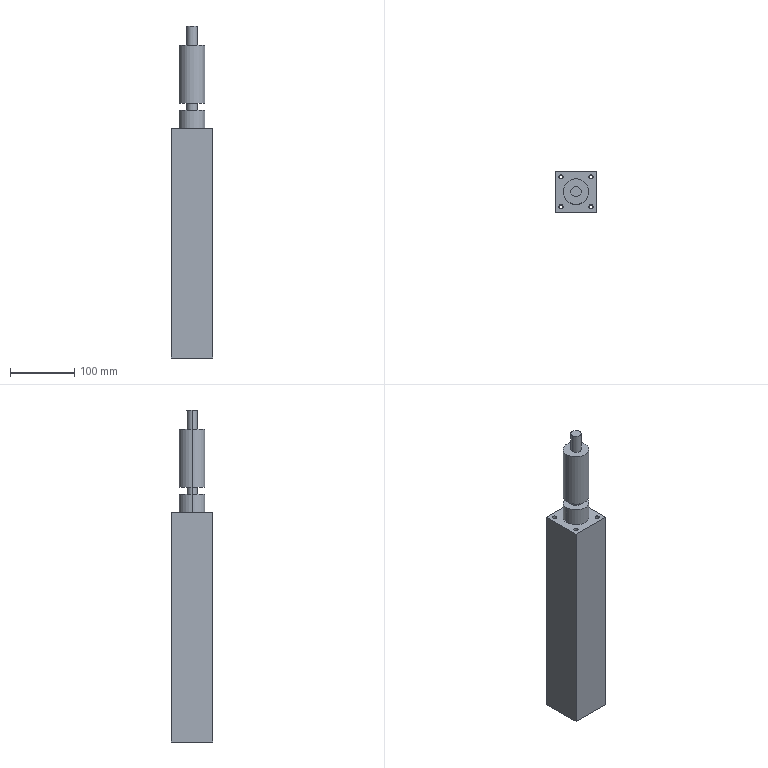Part | 1 solid | 26 faces | box 64 x 64 x 515 mm | volume 1562988 mm3 | cylinder 16 | plane 10 | commonest cylinder face diameters 6.8 x8 16 x4 40 x4
STEP:
#1=CARTESIAN_POINT('',(8.,0.,337.));
#2=VERTEX_POINT('',#1);
#3=CARTESIAN_POINT('',(-8.,0.,337.));
#4=VERTEX_POINT('',#3);
#5=CARTESIAN_POINT('',(0.,0.,337.));
#6=DIRECTION('',(0.,0.,1.));
#7=DIRECTION('',(1.,0.,0.));
#8=AXIS2_PLACEMENT_3D('',#5,#6,#7);
#9=CIRCLE('',#8,8.);
#10=EDGE_CURVE('',#2,#4,#9,.T.);
#11=ORIENTED_EDGE('',*,*,#10,.F.);
#12=CARTESIAN_POINT('',(8.,0.,307.));
#13=VERTEX_POINT('',#12);
#14=CARTESIAN_POINT('',(8.,0.,337.));
#15=DIRECTION('',(0.,0.,-1.));
#16=VECTOR('',#15,1000.);
#17=LINE('',#14,#16);
#18=EDGE_CURVE('',#2,#13,#17,.T.);
#19=ORIENTED_EDGE('',*,*,#18,.T.);
#20=CARTESIAN_POINT('',(-8.,0.,307.));
#21=VERTEX_POINT('',#20);
#22=CARTESIAN_POINT('',(0.,0.,307.));
#23=DIRECTION('',(0.,0.,1.));
#24=DIRECTION('',(1.,0.,0.));
#25=AXIS2_PLACEMENT_3D('',#22,#23,#24);
#26=CIRCLE('',#25,8.);
#27=EDGE_CURVE('',#13,#21,#26,.T.);
#28=ORIENTED_EDGE('',*,*,#27,.T.);
#29=CARTESIAN_POINT('',(-8.,0.,337.));
#30=DIRECTION('',(0.,0.,-1.));
#31=VECTOR('',#30,1000.);
#32=LINE('',#29,#31);
#33=EDGE_CURVE('',#4,#21,#32,.T.);
#34=ORIENTED_EDGE('',*,*,#33,.F.);
#35=EDGE_LOOP('',(#11,#19,#28,#34));
#36=FACE_OUTER_BOUND('',#35,.T.);
#37=CARTESIAN_POINT('',(0.,0.,337.));
#38=DIRECTION('',(0.,0.,-1.));
#39=DIRECTION('',(-1.,0.,0.));
#40=AXIS2_PLACEMENT_3D('',#37,#38,#39);
#41=CYLINDRICAL_SURFACE('',#40,8.);
#42=ADVANCED_FACE('',(#36),#41,.T.);
#43=CARTESIAN_POINT('',(20.,0.,217.));
#44=VERTEX_POINT('',#43);
#45=CARTESIAN_POINT('',(-20.,0.,217.));
#46=VERTEX_POINT('',#45);
#47=CARTESIAN_POINT('',(0.,0.,217.));
#48=DIRECTION('',(0.,0.,1.));
#49=DIRECTION('',(1.,0.,0.));
#50=AXIS2_PLACEMENT_3D('',#47,#48,#49);
#51=CIRCLE('',#50,20.);
#52=EDGE_CURVE('',#44,#46,#51,.T.);
#53=ORIENTED_EDGE('',*,*,#52,.T.);
#54=CARTESIAN_POINT('',(-20.,0.,307.));
#55=VERTEX_POINT('',#54);
#56=CARTESIAN_POINT('',(-20.,0.,217.));
#57=DIRECTION('',(0.,0.,1.));
#58=VECTOR('',#57,1000.);
#59=LINE('',#56,#58);
#60=EDGE_CURVE('',#46,#55,#59,.T.);
#61=ORIENTED_EDGE('',*,*,#60,.T.);
#62=CARTESIAN_POINT('',(20.,0.,307.));
#63=VERTEX_POINT('',#62);
#64=CARTESIAN_POINT('',(0.,0.,307.));
#65=DIRECTION('',(0.,0.,1.));
#66=DIRECTION('',(1.,0.,0.));
#67=AXIS2_PLACEMENT_3D('',#64,#65,#66);
#68=CIRCLE('',#67,20.);
#69=EDGE_CURVE('',#63,#55,#68,.T.);
#70=ORIENTED_EDGE('',*,*,#69,.F.);
#71=CARTESIAN_POINT('',(20.,0.,217.));
#72=DIRECTION('',(0.,0.,1.));
#73=VECTOR('',#72,1000.);
#74=LINE('',#71,#73);
#75=EDGE_CURVE('',#44,#63,#74,.T.);
#76=ORIENTED_EDGE('',*,*,#75,.F.);
#77=EDGE_LOOP('',(#53,#61,#70,#76));
#78=FACE_OUTER_BOUND('',#77,.T.);
#79=CARTESIAN_POINT('',(0.,0.,217.));
#80=DIRECTION('',(0.,0.,1.));
#81=DIRECTION('',(1.,0.,0.));
#82=AXIS2_PLACEMENT_3D('',#79,#80,#81);
#83=CYLINDRICAL_SURFACE('',#82,20.);
#84=ADVANCED_FACE('',(#78),#83,.T.);
#85=CARTESIAN_POINT('',(20.,0.,206.));
#86=VERTEX_POINT('',#85);
#87=CARTESIAN_POINT('',(-20.,0.,206.));
#88=VERTEX_POINT('',#87);
#89=CARTESIAN_POINT('',(0.,0.,206.));
#90=DIRECTION('',(0.,0.,1.));
#91=DIRECTION('',(1.,0.,0.));
#92=AXIS2_PLACEMENT_3D('',#89,#90,#91);
#93=CIRCLE('',#92,20.);
#94=EDGE_CURVE('',#86,#88,#93,.T.);
#95=ORIENTED_EDGE('',*,*,#94,.F.);
#96=CARTESIAN_POINT('',(20.,0.,178.));
#97=VERTEX_POINT('',#96);
#98=CARTESIAN_POINT('',(20.,0.,206.));
#99=DIRECTION('',(0.,0.,-1.));
#100=VECTOR('',#99,1000.);
#101=LINE('',#98,#100);
#102=EDGE_CURVE('',#86,#97,#101,.T.);
#103=ORIENTED_EDGE('',*,*,#102,.T.);
#104=CARTESIAN_POINT('',(-20.,0.,178.));
#105=VERTEX_POINT('',#104);
#106=CARTESIAN_POINT('',(0.,0.,178.));
#107=DIRECTION('',(0.,0.,1.));
#108=DIRECTION('',(1.,0.,0.));
#109=AXIS2_PLACEMENT_3D('',#106,#107,#108);
#110=CIRCLE('',#109,20.);
#111=EDGE_CURVE('',#97,#105,#110,.T.);
#112=ORIENTED_EDGE('',*,*,#111,.T.);
#113=CARTESIAN_POINT('',(-20.,0.,206.));
#114=DIRECTION('',(0.,0.,-1.));
#115=VECTOR('',#114,1000.);
#116=LINE('',#113,#115);
#117=EDGE_CURVE('',#88,#105,#116,.T.);
#118=ORIENTED_EDGE('',*,*,#117,.F.);
#119=EDGE_LOOP('',(#95,#103,#112,#118));
#120=FACE_OUTER_BOUND('',#119,.T.);
#121=CARTESIAN_POINT('',(0.,0.,206.));
#122=DIRECTION('',(0.,0.,-1.));
#123=DIRECTION('',(-1.,0.,0.));
#124=AXIS2_PLACEMENT_3D('',#121,#122,#123);
#125=CYLINDRICAL_SURFACE('',#124,20.);
#126=ADVANCED_FACE('',(#120),#125,.T.);
#127=CARTESIAN_POINT('',(-26.65,23.25,-178.));
#128=VERTEX_POINT('',#127);
#129=CARTESIAN_POINT('',(-19.85,23.25,-178.));
#130=VERTEX_POINT('',#129);
#131=CARTESIAN_POINT('',(-23.25,23.25,-178.));
#132=DIRECTION('',(0.,0.,1.));
#133=DIRECTION('',(1.,0.,0.));
#134=AXIS2_PLACEMENT_3D('',#131,#132,#133);
#135=CIRCLE('',#134,3.4);
#136=EDGE_CURVE('',#128,#130,#135,.T.);
#137=ORIENTED_EDGE('',*,*,#136,.F.);
#138=CARTESIAN_POINT('',(-26.65,23.25,178.));
#139=VERTEX_POINT('',#138);
#140=CARTESIAN_POINT('',(-26.65,23.25,178.));
#141=DIRECTION('',(0.,0.,1.));
#142=VECTOR('',#141,1000.);
#143=LINE('',#140,#142);
#144=EDGE_CURVE('',#128,#139,#143,.T.);
#145=ORIENTED_EDGE('',*,*,#144,.T.);
#146=CARTESIAN_POINT('',(-19.85,23.25,178.));
#147=VERTEX_POINT('',#146);
#148=CARTESIAN_POINT('',(-23.25,23.25,178.));
#149=DIRECTION('',(0.,0.,1.));
#150=DIRECTION('',(1.,0.,0.));
#151=AXIS2_PLACEMENT_3D('',#148,#149,#150);
#152=CIRCLE('',#151,3.4);
#153=EDGE_CURVE('',#139,#147,#152,.T.);
#154=ORIENTED_EDGE('',*,*,#153,.T.);
#155=CARTESIAN_POINT('',(-19.85,23.25,178.));
#156=DIRECTION('',(0.,0.,1.));
#157=VECTOR('',#156,1000.);
#158=LINE('',#155,#157);
#159=EDGE_CURVE('',#130,#147,#158,.T.);
#160=ORIENTED_EDGE('',*,*,#159,.F.);
#161=EDGE_LOOP('',(#137,#145,#154,#160));
#162=FACE_OUTER_BOUND('',#161,.T.);
#163=CARTESIAN_POINT('',(-23.25,23.25,178.));
#164=DIRECTION('',(0.,0.,1.));
#165=DIRECTION('',(1.,0.,0.));
#166=AXIS2_PLACEMENT_3D('',#163,#164,#165);
#167=CYLINDRICAL_SURFACE('',#166,3.4);
#168=ADVANCED_FACE('',(#162),#167,.F.);
#169=CARTESIAN_POINT('',(19.85,23.25,-178.));
#170=VERTEX_POINT('',#169);
#171=CARTESIAN_POINT('',(26.65,23.25,-178.));
#172=VERTEX_POINT('',#171);
#173=CARTESIAN_POINT('',(23.25,23.25,-178.));
#174=DIRECTION('',(0.,0.,1.));
#175=DIRECTION('',(1.,0.,0.));
#176=AXIS2_PLACEMENT_3D('',#173,#174,#175);
#177=CIRCLE('',#176,3.4);
#178=EDGE_CURVE('',#170,#172,#177,.T.);
#179=ORIENTED_EDGE('',*,*,#178,.F.);
#180=CARTESIAN_POINT('',(19.85,23.25,178.));
#181=VERTEX_POINT('',#180);
#182=CARTESIAN_POINT('',(19.85,23.25,178.));
#183=DIRECTION('',(0.,0.,1.));
#184=VECTOR('',#183,1000.);
#185=LINE('',#182,#184);
#186=EDGE_CURVE('',#170,#181,#185,.T.);
#187=ORIENTED_EDGE('',*,*,#186,.T.);
#188=CARTESIAN_POINT('',(26.65,23.25,178.));
#189=VERTEX_POINT('',#188);
#190=CARTESIAN_POINT('',(23.25,23.25,178.));
#191=DIRECTION('',(0.,0.,1.));
#192=DIRECTION('',(1.,0.,0.));
#193=AXIS2_PLACEMENT_3D('',#190,#191,#192);
#194=CIRCLE('',#193,3.4);
#195=EDGE_CURVE('',#181,#189,#194,.T.);
#196=ORIENTED_EDGE('',*,*,#195,.T.);
#197=CARTESIAN_POINT('',(26.65,23.25,178.));
#198=DIRECTION('',(0.,0.,1.));
#199=VECTOR('',#198,1000.);
#200=LINE('',#197,#199);
#201=EDGE_CURVE('',#172,#189,#200,.T.);
#202=ORIENTED_EDGE('',*,*,#201,.F.);
#203=EDGE_LOOP('',(#179,#187,#196,#202));
#204=FACE_OUTER_BOUND('',#203,.T.);
#205=CARTESIAN_POINT('',(23.25,23.25,178.));
#206=DIRECTION('',(0.,0.,1.));
#207=DIRECTION('',(1.,0.,0.));
#208=AXIS2_PLACEMENT_3D('',#205,#206,#207);
#209=CYLINDRICAL_SURFACE('',#208,3.4);
#210=ADVANCED_FACE('',(#204),#209,.F.);
#211=CARTESIAN_POINT('',(19.85,-23.25,-178.));
#212=VERTEX_POINT('',#211);
#213=CARTESIAN_POINT('',(26.65,-23.25,-178.));
#214=VERTEX_POINT('',#213);
#215=CARTESIAN_POINT('',(23.25,-23.25,-178.));
#216=DIRECTION('',(0.,0.,1.));
#217=DIRECTION('',(1.,0.,0.));
#218=AXIS2_PLACEMENT_3D('',#215,#216,#217);
#219=CIRCLE('',#218,3.4);
#220=EDGE_CURVE('',#212,#214,#219,.T.);
#221=ORIENTED_EDGE('',*,*,#220,.F.);
#222=CARTESIAN_POINT('',(19.85,-23.25,178.));
#223=VERTEX_POINT('',#222);
#224=CARTESIAN_POINT('',(19.85,-23.25,178.));
#225=DIRECTION('',(0.,0.,1.));
#226=VECTOR('',#225,1000.);
#227=LINE('',#224,#226);
#228=EDGE_CURVE('',#212,#223,#227,.T.);
#229=ORIENTED_EDGE('',*,*,#228,.T.);
#230=CARTESIAN_POINT('',(26.65,-23.25,178.));
#231=VERTEX_POINT('',#230);
#232=CARTESIAN_POINT('',(23.25,-23.25,178.));
#233=DIRECTION('',(0.,0.,1.));
#234=DIRECTION('',(1.,0.,0.));
#235=AXIS2_PLACEMENT_3D('',#232,#233,#234);
#236=CIRCLE('',#235,3.4);
#237=EDGE_CURVE('',#223,#231,#236,.T.);
#238=ORIENTED_EDGE('',*,*,#237,.T.);
#239=CARTESIAN_POINT('',(26.65,-23.25,178.));
#240=DIRECTION('',(0.,0.,1.));
#241=VECTOR('',#240,1000.);
#242=LINE('',#239,#241);
#243=EDGE_CURVE('',#214,#231,#242,.T.);
#244=ORIENTED_EDGE('',*,*,#243,.F.);
#245=EDGE_LOOP('',(#221,#229,#238,#244));
#246=FACE_OUTER_BOUND('',#245,.T.);
#247=CARTESIAN_POINT('',(23.25,-23.25,178.));
#248=DIRECTION('',(0.,0.,1.));
#249=DIRECTION('',(1.,0.,0.));
#250=AXIS2_PLACEMENT_3D('',#247,#248,#249);
#251=CYLINDRICAL_SURFACE('',#250,3.4);
#252=ADVANCED_FACE('',(#246),#251,.F.);
#253=CARTESIAN_POINT('',(-26.65,-23.25,-178.));
#254=VERTEX_POINT('',#253);
#255=CARTESIAN_POINT('',(-19.85,-23.25,-178.));
#256=VERTEX_POINT('',#255);
#257=CARTESIAN_POINT('',(-23.25,-23.25,-178.));
#258=DIRECTION('',(0.,0.,1.));
#259=DIRECTION('',(1.,0.,0.));
#260=AXIS2_PLACEMENT_3D('',#257,#258,#259);
#261=CIRCLE('',#260,3.4);
#262=EDGE_CURVE('',#254,#256,#261,.T.);
#263=ORIENTED_EDGE('',*,*,#262,.F.);
#264=CARTESIAN_POINT('',(-26.65,-23.25,178.));
#265=VERTEX_POINT('',#264);
#266=CARTESIAN_POINT('',(-26.65,-23.25,178.));
#267=DIRECTION('',(0.,0.,1.));
#268=VECTOR('',#267,1000.);
#269=LINE('',#266,#268);
#270=EDGE_CURVE('',#254,#265,#269,.T.);
#271=ORIENTED_EDGE('',*,*,#270,.T.);
#272=CARTESIAN_POINT('',(-19.85,-23.25,178.));
#273=VERTEX_POINT('',#272);
#274=CARTESIAN_POINT('',(-23.25,-23.25,178.));
#275=DIRECTION('',(0.,0.,1.));
#276=DIRECTION('',(1.,0.,0.));
#277=AXIS2_PLACEMENT_3D('',#274,#275,#276);
#278=CIRCLE('',#277,3.4);
#279=EDGE_CURVE('',#265,#273,#278,.T.);
#280=ORIENTED_EDGE('',*,*,#279,.T.);
#281=CARTESIAN_POINT('',(-19.85,-23.25,178.));
#282=DIRECTION('',(0.,0.,1.));
#283=VECTOR('',#282,1000.);
#284=LINE('',#281,#283);
#285=EDGE_CURVE('',#256,#273,#284,.T.);
#286=ORIENTED_EDGE('',*,*,#285,.F.);
#287=EDGE_LOOP('',(#263,#271,#280,#286));
#288=FACE_OUTER_BOUND('',#287,.T.);
#289=CARTESIAN_POINT('',(-23.25,-23.25,178.));
#290=DIRECTION('',(0.,0.,1.));
#291=DIRECTION('',(1.,0.,0.));
#292=AXIS2_PLACEMENT_3D('',#289,#290,#291);
#293=CYLINDRICAL_SURFACE('',#292,3.4);
#294=ADVANCED_FACE('',(#288),#293,.F.);
#295=CARTESIAN_POINT('',(8.,0.,217.));
#296=VERTEX_POINT('',#295);
#297=CARTESIAN_POINT('',(-8.,0.,217.));
#298=VERTEX_POINT('',#297);
#299=CARTESIAN_POINT('',(0.,0.,217.));
#300=DIRECTION('',(0.,0.,1.));
#301=DIRECTION('',(1.,0.,0.));
#302=AXIS2_PLACEMENT_3D('',#299,#300,#301);
#303=CIRCLE('',#302,8.);
#304=EDGE_CURVE('',#296,#298,#303,.T.);
#305=ORIENTED_EDGE('',*,*,#304,.F.);
#306=CARTESIAN_POINT('',(8.,0.,206.));
#307=VERTEX_POINT('',#306);
#308=CARTESIAN_POINT('',(8.,0.,247.));
#309=DIRECTION('',(0.,0.,-1.));
#310=VECTOR('',#309,1000.);
#311=LINE('',#308,#310);
#312=EDGE_CURVE('',#296,#307,#311,.T.);
#313=ORIENTED_EDGE('',*,*,#312,.T.);
#314=CARTESIAN_POINT('',(-8.,0.,206.));
#315=VERTEX_POINT('',#314);
#316=CARTESIAN_POINT('',(0.,0.,206.));
#317=DIRECTION('',(0.,0.,1.));
#318=DIRECTION('',(1.,0.,0.));
#319=AXIS2_PLACEMENT_3D('',#316,#317,#318);
#320=CIRCLE('',#319,8.);
#321=EDGE_CURVE('',#307,#315,#320,.T.);
#322=ORIENTED_EDGE('',*,*,#321,.T.);
#323=CARTESIAN_POINT('',(-8.,0.,247.));
#324=DIRECTION('',(0.,0.,-1.));
#325=VECTOR('',#324,1000.);
#326=LINE('',#323,#325);
#327=EDGE_CURVE('',#298,#315,#326,.T.);
#328=ORIENTED_EDGE('',*,*,#327,.F.);
#329=EDGE_LOOP('',(#305,#313,#322,#328));
#330=FACE_OUTER_BOUND('',#329,.T.);
#331=CARTESIAN_POINT('',(0.,0.,247.));
#332=DIRECTION('',(0.,0.,-1.));
#333=DIRECTION('',(-1.,0.,0.));
#334=AXIS2_PLACEMENT_3D('',#331,#332,#333);
#335=CYLINDRICAL_SURFACE('',#334,8.);
#336=ADVANCED_FACE('',(#330),#335,.T.);
#337=ORIENTED_EDGE('',*,*,#312,.F.);
#338=CARTESIAN_POINT('',(0.,0.,217.));
#339=DIRECTION('',(0.,0.,1.));
#340=DIRECTION('',(1.,0.,0.));
#341=AXIS2_PLACEMENT_3D('',#338,#339,#340);
#342=CIRCLE('',#341,8.);
#343=EDGE_CURVE('',#298,#296,#342,.T.);
#344=ORIENTED_EDGE('',*,*,#343,.F.);
#345=ORIENTED_EDGE('',*,*,#327,.T.);
#346=CARTESIAN_POINT('',(0.,0.,206.));
#347=DIRECTION('',(0.,0.,1.));
#348=DIRECTION('',(1.,0.,0.));
#349=AXIS2_PLACEMENT_3D('',#346,#347,#348);
#350=CIRCLE('',#349,8.);
#351=EDGE_CURVE('',#315,#307,#350,.T.);
#352=ORIENTED_EDGE('',*,*,#351,.T.);
#353=EDGE_LOOP('',(#337,#344,#345,#352));
#354=FACE_OUTER_BOUND('',#353,.T.);
#355=CARTESIAN_POINT('',(0.,0.,247.));
#356=DIRECTION('',(0.,0.,-1.));
#357=DIRECTION('',(-1.,0.,0.));
#358=AXIS2_PLACEMENT_3D('',#355,#356,#357);
#359=CYLINDRICAL_SURFACE('',#358,8.);
#360=ADVANCED_FACE('',(#354),#359,.T.);
#361=CARTESIAN_POINT('',(-32.,32.,-178.));
#362=VERTEX_POINT('',#361);
#363=CARTESIAN_POINT('',(-32.,-32.,-178.));
#364=VERTEX_POINT('',#363);
#365=CARTESIAN_POINT('',(-32.,32.,-178.));
#366=DIRECTION('',(0.,-1.,0.));
#367=VECTOR('',#366,1000.);
#368=LINE('',#365,#367);
#369=EDGE_CURVE('',#362,#364,#368,.T.);
#370=ORIENTED_EDGE('',*,*,#369,.T.);
#371=CARTESIAN_POINT('',(-32.,-32.,178.));
#372=VERTEX_POINT('',#371);
#373=CARTESIAN_POINT('',(-32.,-32.,178.));
#374=DIRECTION('',(0.,0.,-1.));
#375=VECTOR('',#374,1000.);
#376=LINE('',#373,#375);
#377=EDGE_CURVE('',#372,#364,#376,.T.);
#378=ORIENTED_EDGE('',*,*,#377,.F.);
#379=CARTESIAN_POINT('',(-32.,32.,178.));
#380=VERTEX_POINT('',#379);
#381=CARTESIAN_POINT('',(-32.,32.,178.));
#382=DIRECTION('',(0.,-1.,0.));
#383=VECTOR('',#382,1000.);
#384=LINE('',#381,#383);
#385=EDGE_CURVE('',#380,#372,#384,.T.);
#386=ORIENTED_EDGE('',*,*,#385,.F.);
#387=CARTESIAN_POINT('',(-32.,32.,178.));
#388=DIRECTION('',(0.,0.,-1.));
#389=VECTOR('',#388,1000.);
#390=LINE('',#387,#389);
#391=EDGE_CURVE('',#380,#362,#390,.T.);
#392=ORIENTED_EDGE('',*,*,#391,.T.);
#393=EDGE_LOOP('',(#370,#378,#386,#392));
#394=FACE_OUTER_BOUND('',#393,.T.);
#395=CARTESIAN_POINT('',(-32.,32.,178.));
#396=DIRECTION('',(1.,0.,0.));
#397=DIRECTION('',(0.,1.,0.));
#398=AXIS2_PLACEMENT_3D('',#395,#396,#397);
#399=PLANE('',#398);
#400=ADVANCED_FACE('',(#394),#399,.F.);
#401=CARTESIAN_POINT('',(32.,-32.,-178.));
#402=VERTEX_POINT('',#401);
#403=CARTESIAN_POINT('',(-32.,-32.,-178.));
#404=DIRECTION('',(1.,0.,0.));
#405=VECTOR('',#404,1000.);
#406=LINE('',#403,#405);
#407=EDGE_CURVE('',#364,#402,#406,.T.);
#408=ORIENTED_EDGE('',*,*,#407,.T.);
#409=CARTESIAN_POINT('',(32.,-32.,178.));
#410=VERTEX_POINT('',#409);
#411=CARTESIAN_POINT('',(32.,-32.,178.));
#412=DIRECTION('',(0.,0.,-1.));
#413=VECTOR('',#412,1000.);
#414=LINE('',#411,#413);
#415=EDGE_CURVE('',#410,#402,#414,.T.);
#416=ORIENTED_EDGE('',*,*,#415,.F.);
#417=CARTESIAN_POINT('',(-32.,-32.,178.));
#418=DIRECTION('',(1.,0.,0.));
#419=VECTOR('',#418,1000.);
#420=LINE('',#417,#419);
#421=EDGE_CURVE('',#372,#410,#420,.T.);
#422=ORIENTED_EDGE('',*,*,#421,.F.);
#423=ORIENTED_EDGE('',*,*,#377,.T.);
#424=EDGE_LOOP('',(#408,#416,#422,#423));
#425=FACE_OUTER_BOUND('',#424,.T.);
#426=CARTESIAN_POINT('',(-32.,-32.,178.));
#427=DIRECTION('',(0.,1.,0.));
#428=DIRECTION('',(0.,0.,1.));
#429=AXIS2_PLACEMENT_3D('',#426,#427,#428);
#430=PLANE('',#429);
#431=ADVANCED_FACE('',(#425),#430,.F.);
#432=CARTESIAN_POINT('',(32.,32.,-178.));
#433=VERTEX_POINT('',#432);
#434=CARTESIAN_POINT('',(32.,32.,-178.));
#435=DIRECTION('',(0.,1.,0.));
#436=VECTOR('',#435,1000.);
#437=LINE('',#434,#436);
#438=EDGE_CURVE('',#402,#433,#437,.T.);
#439=ORIENTED_EDGE('',*,*,#438,.T.);
#440=CARTESIAN_POINT('',(32.,32.,178.));
#441=VERTEX_POINT('',#440);
#442=CARTESIAN_POINT('',(32.,32.,178.));
#443=DIRECTION('',(0.,0.,-1.));
#444=VECTOR('',#443,1000.);
#445=LINE('',#442,#444);
#446=EDGE_CURVE('',#441,#433,#445,.T.);
#447=ORIENTED_EDGE('',*,*,#446,.F.);
#448=CARTESIAN_POINT('',(32.,32.,178.));
#449=DIRECTION('',(0.,1.,0.));
#450=VECTOR('',#449,1000.);
#451=LINE('',#448,#450);
#452=EDGE_CURVE('',#410,#441,#451,.T.);
#453=ORIENTED_EDGE('',*,*,#452,.F.);
#454=ORIENTED_EDGE('',*,*,#415,.T.);
#455=EDGE_LOOP('',(#439,#447,#453,#454));
#456=FACE_OUTER_BOUND('',#455,.T.);
#457=CARTESIAN_POINT('',(32.,32.,178.));
#458=DIRECTION('',(-1.,0.,0.));
#459=DIRECTION('',(0.,-1.,0.));
#460=AXIS2_PLACEMENT_3D('',#457,#458,#459);
#461=PLANE('',#460);
#462=ADVANCED_FACE('',(#456),#461,.F.);
#463=CARTESIAN_POINT('',(-32.,32.,-178.));
#464=DIRECTION('',(-1.,0.,0.));
#465=VECTOR('',#464,1000.);
#466=LINE('',#463,#465);
#467=EDGE_CURVE('',#433,#362,#466,.T.);
#468=ORIENTED_EDGE('',*,*,#467,.T.);
#469=ORIENTED_EDGE('',*,*,#391,.F.);
#470=CARTESIAN_POINT('',(-32.,32.,178.));
#471=DIRECTION('',(-1.,0.,0.));
#472=VECTOR('',#471,1000.);
#473=LINE('',#470,#472);
#474=EDGE_CURVE('',#441,#380,#473,.T.);
#475=ORIENTED_EDGE('',*,*,#474,.F.);
#476=ORIENTED_EDGE('',*,*,#446,.T.);
#477=EDGE_LOOP('',(#468,#469,#475,#476));
#478=FACE_OUTER_BOUND('',#477,.T.);
#479=CARTESIAN_POINT('',(-32.,32.,178.));
#480=DIRECTION('',(0.,-1.,0.));
#481=DIRECTION('',(0.,0.,-1.));
#482=AXIS2_PLACEMENT_3D('',#479,#480,#481);
#483=PLANE('',#482);
#484=ADVANCED_FACE('',(#478),#483,.F.);
#485=CARTESIAN_POINT('',(0.,0.,178.));
#486=DIRECTION('',(0.,0.,1.));
#487=DIRECTION('',(1.,0.,0.));
#488=AXIS2_PLACEMENT_3D('',#485,#486,#487);
#489=CIRCLE('',#488,20.);
#490=EDGE_CURVE('',#105,#97,#489,.T.);
#491=ORIENTED_EDGE('',*,*,#490,.F.);
#492=ORIENTED_EDGE('',*,*,#111,.F.);
#493=EDGE_LOOP('',(#491,#492));
#494=FACE_BOUND('',#493,.T.);
#495=CARTESIAN_POINT('',(-23.25,23.25,178.));
#496=DIRECTION('',(0.,0.,1.));
#497=DIRECTION('',(1.,0.,0.));
#498=AXIS2_PLACEMENT_3D('',#495,#496,#497);
#499=CIRCLE('',#498,3.4);
#500=EDGE_CURVE('',#147,#139,#499,.T.);
#501=ORIENTED_EDGE('',*,*,#500,.F.);
#502=ORIENTED_EDGE('',*,*,#153,.F.);
#503=EDGE_LOOP('',(#501,#502));
#504=FACE_BOUND('',#503,.T.);
#505=CARTESIAN_POINT('',(23.25,23.25,178.));
#506=DIRECTION('',(0.,0.,1.));
#507=DIRECTION('',(1.,0.,0.));
#508=AXIS2_PLACEMENT_3D('',#505,#506,#507);
#509=CIRCLE('',#508,3.4);
#510=EDGE_CURVE('',#189,#181,#509,.T.);
#511=ORIENTED_EDGE('',*,*,#510,.F.);
#512=ORIENTED_EDGE('',*,*,#195,.F.);
#513=EDGE_LOOP('',(#511,#512));
#514=FACE_BOUND('',#513,.T.);
#515=CARTESIAN_POINT('',(23.25,-23.25,178.));
#516=DIRECTION('',(0.,0.,1.));
#517=DIRECTION('',(1.,0.,0.));
#518=AXIS2_PLACEMENT_3D('',#515,#516,#517);
#519=CIRCLE('',#518,3.4);
#520=EDGE_CURVE('',#231,#223,#519,.T.);
#521=ORIENTED_EDGE('',*,*,#520,.F.);
#522=ORIENTED_EDGE('',*,*,#237,.F.);
#523=EDGE_LOOP('',(#521,#522));
#524=FACE_BOUND('',#523,.T.);
#525=CARTESIAN_POINT('',(-23.25,-23.25,178.));
#526=DIRECTION('',(0.,0.,1.));
#527=DIRECTION('',(1.,0.,0.));
#528=AXIS2_PLACEMENT_3D('',#525,#526,#527);
#529=CIRCLE('',#528,3.4);
#530=EDGE_CURVE('',#273,#265,#529,.T.);
#531=ORIENTED_EDGE('',*,*,#530,.F.);
#532=ORIENTED_EDGE('',*,*,#279,.F.);
#533=EDGE_LOOP('',(#531,#532));
#534=FACE_BOUND('',#533,.T.);
#535=ORIENTED_EDGE('',*,*,#385,.T.);
#536=ORIENTED_EDGE('',*,*,#421,.T.);
#537=ORIENTED_EDGE('',*,*,#452,.T.);
#538=ORIENTED_EDGE('',*,*,#474,.T.);
#539=EDGE_LOOP('',(#535,#536,#537,#538));
#540=FACE_OUTER_BOUND('',#539,.T.);
#541=CARTESIAN_POINT('',(0.,0.,178.));
#542=DIRECTION('',(0.,0.,1.));
#543=DIRECTION('',(1.,0.,0.));
#544=AXIS2_PLACEMENT_3D('',#541,#542,#543);
#545=PLANE('',#544);
#546=ADVANCED_FACE('',(#494,#504,#514,#524,#534,#540),#545,.T.);
#547=CARTESIAN_POINT('',(-23.25,23.25,-178.));
#548=DIRECTION('',(0.,0.,1.));
#549=DIRECTION('',(1.,0.,0.));
#550=AXIS2_PLACEMENT_3D('',#547,#548,#549);
#551=CIRCLE('',#550,3.4);
#552=EDGE_CURVE('',#130,#128,#551,.T.);
#553=ORIENTED_EDGE('',*,*,#552,.T.);
#554=ORIENTED_EDGE('',*,*,#136,.T.);
#555=EDGE_LOOP('',(#553,#554));
#556=FACE_BOUND('',#555,.T.);
#557=CARTESIAN_POINT('',(23.25,23.25,-178.));
#558=DIRECTION('',(0.,0.,1.));
#559=DIRECTION('',(1.,0.,0.));
#560=AXIS2_PLACEMENT_3D('',#557,#558,#559);
#561=CIRCLE('',#560,3.4);
#562=EDGE_CURVE('',#172,#170,#561,.T.);
#563=ORIENTED_EDGE('',*,*,#562,.T.);
#564=ORIENTED_EDGE('',*,*,#178,.T.);
#565=EDGE_LOOP('',(#563,#564));
#566=FACE_BOUND('',#565,.T.);
#567=CARTESIAN_POINT('',(23.25,-23.25,-178.));
#568=DIRECTION('',(0.,0.,1.));
#569=DIRECTION('',(1.,0.,0.));
#570=AXIS2_PLACEMENT_3D('',#567,#568,#569);
#571=CIRCLE('',#570,3.4);
#572=EDGE_CURVE('',#214,#212,#571,.T.);
#573=ORIENTED_EDGE('',*,*,#572,.T.);
#574=ORIENTED_EDGE('',*,*,#220,.T.);
#575=EDGE_LOOP('',(#573,#574));
#576=FACE_BOUND('',#575,.T.);
#577=CARTESIAN_POINT('',(-23.25,-23.25,-178.));
#578=DIRECTION('',(0.,0.,1.));
#579=DIRECTION('',(1.,0.,0.));
#580=AXIS2_PLACEMENT_3D('',#577,#578,#579);
#581=CIRCLE('',#580,3.4);
#582=EDGE_CURVE('',#256,#254,#581,.T.);
#583=ORIENTED_EDGE('',*,*,#582,.T.);
#584=ORIENTED_EDGE('',*,*,#262,.T.);
#585=EDGE_LOOP('',(#583,#584));
#586=FACE_BOUND('',#585,.T.);
#587=ORIENTED_EDGE('',*,*,#369,.F.);
#588=ORIENTED_EDGE('',*,*,#467,.F.);
#589=ORIENTED_EDGE('',*,*,#438,.F.);
#590=ORIENTED_EDGE('',*,*,#407,.F.);
#591=EDGE_LOOP('',(#587,#588,#589,#590));
#592=FACE_OUTER_BOUND('',#591,.T.);
#593=CARTESIAN_POINT('',(0.,0.,-178.));
#594=DIRECTION('',(0.,0.,1.));
#595=DIRECTION('',(1.,0.,0.));
#596=AXIS2_PLACEMENT_3D('',#593,#594,#595);
#597=PLANE('',#596);
#598=ADVANCED_FACE('',(#556,#566,#576,#586,#592),#597,.F.);
#599=ORIENTED_EDGE('',*,*,#270,.F.);
#600=ORIENTED_EDGE('',*,*,#582,.F.);
#601=ORIENTED_EDGE('',*,*,#285,.T.);
#602=ORIENTED_EDGE('',*,*,#530,.T.);
#603=EDGE_LOOP('',(#599,#600,#601,#602));
#604=FACE_OUTER_BOUND('',#603,.T.);
#605=CARTESIAN_POINT('',(-23.25,-23.25,178.));
#606=DIRECTION('',(0.,0.,1.));
#607=DIRECTION('',(1.,0.,0.));
#608=AXIS2_PLACEMENT_3D('',#605,#606,#607);
#609=CYLINDRICAL_SURFACE('',#608,3.4);
#610=ADVANCED_FACE('',(#604),#609,.F.);
#611=ORIENTED_EDGE('',*,*,#228,.F.);
#612=ORIENTED_EDGE('',*,*,#572,.F.);
#613=ORIENTED_EDGE('',*,*,#243,.T.);
#614=ORIENTED_EDGE('',*,*,#520,.T.);
#615=EDGE_LOOP('',(#611,#612,#613,#614));
#616=FACE_OUTER_BOUND('',#615,.T.);
#617=CARTESIAN_POINT('',(23.25,-23.25,178.));
#618=DIRECTION('',(0.,0.,1.));
#619=DIRECTION('',(1.,0.,0.));
#620=AXIS2_PLACEMENT_3D('',#617,#618,#619);
#621=CYLINDRICAL_SURFACE('',#620,3.4);
#622=ADVANCED_FACE('',(#616),#621,.F.);
#623=ORIENTED_EDGE('',*,*,#186,.F.);
#624=ORIENTED_EDGE('',*,*,#562,.F.);
#625=ORIENTED_EDGE('',*,*,#201,.T.);
#626=ORIENTED_EDGE('',*,*,#510,.T.);
#627=EDGE_LOOP('',(#623,#624,#625,#626));
#628=FACE_OUTER_BOUND('',#627,.T.);
#629=CARTESIAN_POINT('',(23.25,23.25,178.));
#630=DIRECTION('',(0.,0.,1.));
#631=DIRECTION('',(1.,0.,0.));
#632=AXIS2_PLACEMENT_3D('',#629,#630,#631);
#633=CYLINDRICAL_SURFACE('',#632,3.4);
#634=ADVANCED_FACE('',(#628),#633,.F.);
#635=ORIENTED_EDGE('',*,*,#144,.F.);
#636=ORIENTED_EDGE('',*,*,#552,.F.);
#637=ORIENTED_EDGE('',*,*,#159,.T.);
#638=ORIENTED_EDGE('',*,*,#500,.T.);
#639=EDGE_LOOP('',(#635,#636,#637,#638));
#640=FACE_OUTER_BOUND('',#639,.T.);
#641=CARTESIAN_POINT('',(-23.25,23.25,178.));
#642=DIRECTION('',(0.,0.,1.));
#643=DIRECTION('',(1.,0.,0.));
#644=AXIS2_PLACEMENT_3D('',#641,#642,#643);
#645=CYLINDRICAL_SURFACE('',#644,3.4);
#646=ADVANCED_FACE('',(#640),#645,.F.);
#647=ORIENTED_EDGE('',*,*,#102,.F.);
#648=CARTESIAN_POINT('',(0.,0.,206.));
#649=DIRECTION('',(0.,0.,1.));
#650=DIRECTION('',(1.,0.,0.));
#651=AXIS2_PLACEMENT_3D('',#648,#649,#650);
#652=CIRCLE('',#651,20.);
#653=EDGE_CURVE('',#88,#86,#652,.T.);
#654=ORIENTED_EDGE('',*,*,#653,.F.);
#655=ORIENTED_EDGE('',*,*,#117,.T.);
#656=ORIENTED_EDGE('',*,*,#490,.T.);
#657=EDGE_LOOP('',(#647,#654,#655,#656));
#658=FACE_OUTER_BOUND('',#657,.T.);
#659=CARTESIAN_POINT('',(0.,0.,206.));
#660=DIRECTION('',(0.,0.,-1.));
#661=DIRECTION('',(-1.,0.,0.));
#662=AXIS2_PLACEMENT_3D('',#659,#660,#661);
#663=CYLINDRICAL_SURFACE('',#662,20.);
#664=ADVANCED_FACE('',(#658),#663,.T.);
#665=ORIENTED_EDGE('',*,*,#351,.F.);
#666=ORIENTED_EDGE('',*,*,#321,.F.);
#667=EDGE_LOOP('',(#665,#666));
#668=FACE_BOUND('',#667,.T.);
#669=ORIENTED_EDGE('',*,*,#653,.T.);
#670=ORIENTED_EDGE('',*,*,#94,.T.);
#671=EDGE_LOOP('',(#669,#670));
#672=FACE_OUTER_BOUND('',#671,.T.);
#673=CARTESIAN_POINT('',(0.,0.,206.));
#674=DIRECTION('',(0.,0.,1.));
#675=DIRECTION('',(1.,0.,0.));
#676=AXIS2_PLACEMENT_3D('',#673,#674,#675);
#677=PLANE('',#676);
#678=ADVANCED_FACE('',(#668,#672),#677,.T.);
#679=ORIENTED_EDGE('',*,*,#60,.F.);
#680=CARTESIAN_POINT('',(0.,0.,217.));
#681=DIRECTION('',(0.,0.,1.));
#682=DIRECTION('',(1.,0.,0.));
#683=AXIS2_PLACEMENT_3D('',#680,#681,#682);
#684=CIRCLE('',#683,20.);
#685=EDGE_CURVE('',#46,#44,#684,.T.);
#686=ORIENTED_EDGE('',*,*,#685,.T.);
#687=ORIENTED_EDGE('',*,*,#75,.T.);
#688=CARTESIAN_POINT('',(0.,0.,307.));
#689=DIRECTION('',(0.,0.,1.));
#690=DIRECTION('',(1.,0.,0.));
#691=AXIS2_PLACEMENT_3D('',#688,#689,#690);
#692=CIRCLE('',#691,20.);
#693=EDGE_CURVE('',#55,#63,#692,.T.);
#694=ORIENTED_EDGE('',*,*,#693,.F.);
#695=EDGE_LOOP('',(#679,#686,#687,#694));
#696=FACE_OUTER_BOUND('',#695,.T.);
#697=CARTESIAN_POINT('',(0.,0.,217.));
#698=DIRECTION('',(0.,0.,1.));
#699=DIRECTION('',(1.,0.,0.));
#700=AXIS2_PLACEMENT_3D('',#697,#698,#699);
#701=CYLINDRICAL_SURFACE('',#700,20.);
#702=ADVANCED_FACE('',(#696),#701,.T.);
#703=ORIENTED_EDGE('',*,*,#343,.T.);
#704=ORIENTED_EDGE('',*,*,#304,.T.);
#705=EDGE_LOOP('',(#703,#704));
#706=FACE_BOUND('',#705,.T.);
#707=ORIENTED_EDGE('',*,*,#52,.F.);
#708=ORIENTED_EDGE('',*,*,#685,.F.);
#709=EDGE_LOOP('',(#707,#708));
#710=FACE_OUTER_BOUND('',#709,.T.);
#711=CARTESIAN_POINT('',(0.,0.,217.));
#712=DIRECTION('',(0.,0.,1.));
#713=DIRECTION('',(1.,0.,0.));
#714=AXIS2_PLACEMENT_3D('',#711,#712,#713);
#715=PLANE('',#714);
#716=ADVANCED_FACE('',(#706,#710),#715,.F.);
#717=CARTESIAN_POINT('',(0.,0.,307.));
#718=DIRECTION('',(0.,0.,1.));
#719=DIRECTION('',(1.,0.,0.));
#720=AXIS2_PLACEMENT_3D('',#717,#718,#719);
#721=CIRCLE('',#720,8.);
#722=EDGE_CURVE('',#21,#13,#721,.T.);
#723=ORIENTED_EDGE('',*,*,#722,.F.);
#724=ORIENTED_EDGE('',*,*,#27,.F.);
#725=EDGE_LOOP('',(#723,#724));
#726=FACE_BOUND('',#725,.T.);
#727=ORIENTED_EDGE('',*,*,#69,.T.);
#728=ORIENTED_EDGE('',*,*,#693,.T.);
#729=EDGE_LOOP('',(#727,#728));
#730=FACE_OUTER_BOUND('',#729,.T.);
#731=CARTESIAN_POINT('',(0.,0.,307.));
#732=DIRECTION('',(0.,0.,1.));
#733=DIRECTION('',(1.,0.,0.));
#734=AXIS2_PLACEMENT_3D('',#731,#732,#733);
#735=PLANE('',#734);
#736=ADVANCED_FACE('',(#726,#730),#735,.T.);
#737=ORIENTED_EDGE('',*,*,#18,.F.);
#738=CARTESIAN_POINT('',(0.,0.,337.));
#739=DIRECTION('',(0.,0.,1.));
#740=DIRECTION('',(1.,0.,0.));
#741=AXIS2_PLACEMENT_3D('',#738,#739,#740);
#742=CIRCLE('',#741,8.);
#743=EDGE_CURVE('',#4,#2,#742,.T.);
#744=ORIENTED_EDGE('',*,*,#743,.F.);
#745=ORIENTED_EDGE('',*,*,#33,.T.);
#746=ORIENTED_EDGE('',*,*,#722,.T.);
#747=EDGE_LOOP('',(#737,#744,#745,#746));
#748=FACE_OUTER_BOUND('',#747,.T.);
#749=CARTESIAN_POINT('',(0.,0.,337.));
#750=DIRECTION('',(0.,0.,-1.));
#751=DIRECTION('',(-1.,0.,0.));
#752=AXIS2_PLACEMENT_3D('',#749,#750,#751);
#753=CYLINDRICAL_SURFACE('',#752,8.);
#754=ADVANCED_FACE('',(#748),#753,.T.);
#755=ORIENTED_EDGE('',*,*,#743,.T.);
#756=ORIENTED_EDGE('',*,*,#10,.T.);
#757=EDGE_LOOP('',(#755,#756));
#758=FACE_OUTER_BOUND('',#757,.T.);
#759=CARTESIAN_POINT('',(0.,0.,337.));
#760=DIRECTION('',(0.,0.,1.));
#761=DIRECTION('',(1.,0.,0.));
#762=AXIS2_PLACEMENT_3D('',#759,#760,#761);
#763=PLANE('',#762);
#764=ADVANCED_FACE('',(#758),#763,.T.);
#765=CLOSED_SHELL('',(#42,#84,#126,#168,#210,#252,#294,#336,#360,#400,#431,#462,#484,#546,#598,#610,#622,#634,#646,#664,#678,#702,#716,#736,#754,#764));
#766=MANIFOLD_SOLID_BREP('',#765);
#767=CARTESIAN_POINT('',(0.,0.,0.));
#768=DIRECTION('',(0.,0.,1.));
#769=DIRECTION('',(1.,0.,0.));
#770=AXIS2_PLACEMENT_3D('',#767,#768,#769);
#771=(LENGTH_UNIT()NAMED_UNIT(*)SI_UNIT(.MILLI.,.METRE.));
#772=UNCERTAINTY_MEASURE_WITH_UNIT(LENGTH_MEASURE(0.00001),#771,'','');
#773=(NAMED_UNIT(*)PLANE_ANGLE_UNIT()SI_UNIT($,.RADIAN.));
#774=(NAMED_UNIT(*)SI_UNIT($,.STERADIAN.)SOLID_ANGLE_UNIT());
#775=(GEOMETRIC_REPRESENTATION_CONTEXT(3)GLOBAL_UNCERTAINTY_ASSIGNED_CONTEXT((#772))GLOBAL_UNIT_ASSIGNED_CONTEXT((#771,#773,#774))REPRESENTATION_CONTEXT('',''));
#776=ADVANCED_BREP_SHAPE_REPRESENTATION('',(#766,#770),#775);